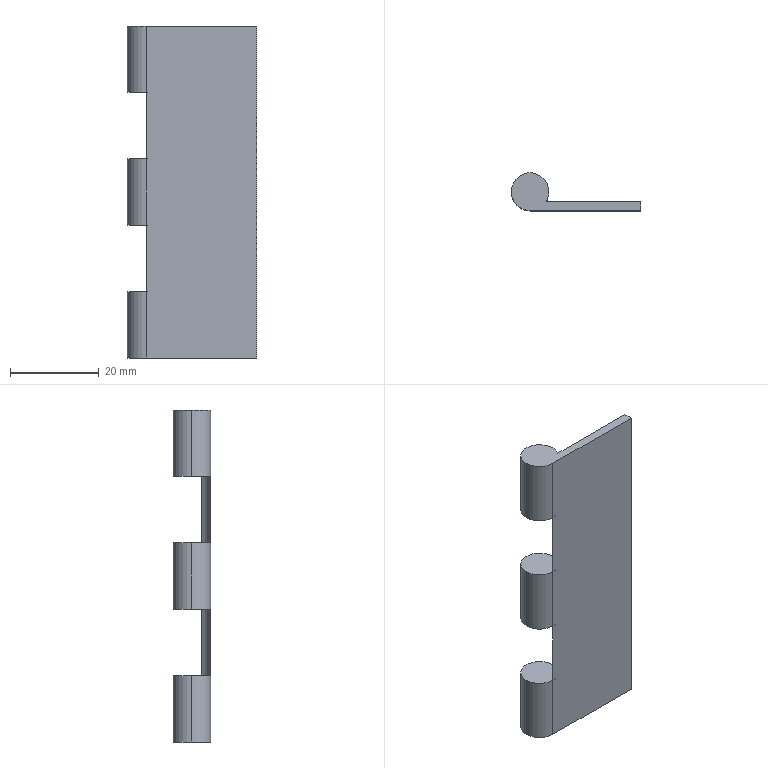Part | STEP file | _PDHFA1-75.step | 1 solid | 20 faces | box 29.25 x 8.5 x 75 mm | volume 5922 mm3 | cylinder 11 | plane 9 | commonest cylinder face diameters 8.5 x11
STEP:
#1=CARTESIAN_POINT('',(0.,0.,0.));
#2=DIRECTION('',(0.,0.,1.));
#3=DIRECTION('',(1.,0.,0.));
#4=AXIS2_PLACEMENT_3D('',#1,#2,#3);
#5=CARTESIAN_POINT('',(3.606,2.,60.));
#6=VERTEX_POINT('',#5);
#7=CARTESIAN_POINT('',(4.25,4.25,60.));
#8=VERTEX_POINT('',#7);
#9=CARTESIAN_POINT('',(0.,4.25,60.));
#10=DIRECTION('',(0.,0.,1.));
#11=DIRECTION('',(1.,0.,0.));
#12=AXIS2_PLACEMENT_3D('',#9,#10,#11);
#13=CIRCLE('',#12,4.25);
#14=CARTESIAN_POINT('',(0.,4.25,75.));
#15=DIRECTION('',(0.,0.,1.));
#16=DIRECTION('',(-1.,0.,0.));
#17=AXIS2_PLACEMENT_3D('',#14,#15,#16);
#18=CYLINDRICAL_SURFACE('',#17,4.25);
#19=CARTESIAN_POINT('',(-3.142,-15.));
#20=DIRECTION('',(1.,0.));
#21=VECTOR('',#20,1.);
#22=LINE('',#19,#21);
#23=(GEOMETRIC_REPRESENTATION_CONTEXT(2)PARAMETRIC_REPRESENTATION_CONTEXT()REPRESENTATION_CONTEXT('',''));
#24=DEFINITIONAL_REPRESENTATION('',(#22),#23);
#25=PCURVE('',#18,#24);
#26=CARTESIAN_POINT('',(0.,4.25,60.));
#27=DIRECTION('',(0.,0.,1.));
#28=DIRECTION('',(1.,0.,0.));
#29=AXIS2_PLACEMENT_3D('',#26,#27,#28);
#30=PLANE('',#29);
#31=CARTESIAN_POINT('',(0.,0.));
#32=DIRECTION('',(1.,0.));
#33=AXIS2_PLACEMENT_2D('',#31,#32);
#34=CIRCLE('',#33,4.25);
#35=(GEOMETRIC_REPRESENTATION_CONTEXT(2)PARAMETRIC_REPRESENTATION_CONTEXT()REPRESENTATION_CONTEXT('',''));
#36=DEFINITIONAL_REPRESENTATION('',(#34),#35);
#37=PCURVE('',#30,#36);
#38=SURFACE_CURVE('',#13,(#25,#37),.PCURVE_S1.);
#39=EDGE_CURVE('',#6,#8,#38,.T.);
#40=ORIENTED_EDGE('',*,*,#39,.T.);
#41=CARTESIAN_POINT('',(4.25,4.25,75.));
#42=VERTEX_POINT('',#41);
#43=CARTESIAN_POINT('',(4.25,4.25,75.));
#44=DIRECTION('',(0.,0.,1.));
#45=VECTOR('',#44,1.);
#46=LINE('',#43,#45);
#47=CARTESIAN_POINT('',(3.142,0.));
#48=DIRECTION('',(0.,1.));
#49=VECTOR('',#48,1.);
#50=LINE('',#47,#49);
#51=(GEOMETRIC_REPRESENTATION_CONTEXT(2)PARAMETRIC_REPRESENTATION_CONTEXT()REPRESENTATION_CONTEXT('',''));
#52=DEFINITIONAL_REPRESENTATION('',(#50),#51);
#53=PCURVE('',#18,#52);
#54=CARTESIAN_POINT('',(0.,4.25,75.));
#55=DIRECTION('',(0.,0.,1.));
#56=DIRECTION('',(-1.,0.,0.));
#57=AXIS2_PLACEMENT_3D('',#54,#55,#56);
#58=CYLINDRICAL_SURFACE('',#57,4.25);
#59=CARTESIAN_POINT('',(3.142,0.));
#60=DIRECTION('',(0.,1.));
#61=VECTOR('',#60,1.);
#62=LINE('',#59,#61);
#63=(GEOMETRIC_REPRESENTATION_CONTEXT(2)PARAMETRIC_REPRESENTATION_CONTEXT()REPRESENTATION_CONTEXT('',''));
#64=DEFINITIONAL_REPRESENTATION('',(#62),#63);
#65=PCURVE('',#58,#64);
#66=SURFACE_CURVE('',#46,(#53,#65),.PCURVE_S1.);
#67=EDGE_CURVE('',#8,#42,#66,.T.);
#68=ORIENTED_EDGE('',*,*,#67,.T.);
#69=CARTESIAN_POINT('',(3.606,2.,75.));
#70=VERTEX_POINT('',#69);
#71=CARTESIAN_POINT('',(0.,4.25,75.));
#72=DIRECTION('',(0.,0.,1.));
#73=DIRECTION('',(1.,0.,0.));
#74=AXIS2_PLACEMENT_3D('',#71,#72,#73);
#75=CIRCLE('',#74,4.25);
#76=CARTESIAN_POINT('',(-3.142,0.));
#77=DIRECTION('',(1.,0.));
#78=VECTOR('',#77,1.);
#79=LINE('',#76,#78);
#80=(GEOMETRIC_REPRESENTATION_CONTEXT(2)PARAMETRIC_REPRESENTATION_CONTEXT()REPRESENTATION_CONTEXT('',''));
#81=DEFINITIONAL_REPRESENTATION('',(#79),#80);
#82=PCURVE('',#18,#81);
#83=CARTESIAN_POINT('',(0.,4.25,75.));
#84=DIRECTION('',(0.,0.,1.));
#85=DIRECTION('',(1.,0.,0.));
#86=AXIS2_PLACEMENT_3D('',#83,#84,#85);
#87=PLANE('',#86);
#88=CARTESIAN_POINT('',(0.,0.));
#89=DIRECTION('',(1.,0.));
#90=AXIS2_PLACEMENT_2D('',#88,#89);
#91=CIRCLE('',#90,4.25);
#92=(GEOMETRIC_REPRESENTATION_CONTEXT(2)PARAMETRIC_REPRESENTATION_CONTEXT()REPRESENTATION_CONTEXT('',''));
#93=DEFINITIONAL_REPRESENTATION('',(#91),#92);
#94=PCURVE('',#87,#93);
#95=SURFACE_CURVE('',#75,(#82,#94),.PCURVE_S1.);
#96=EDGE_CURVE('',#70,#42,#95,.T.);
#97=ORIENTED_EDGE('',*,*,#96,.F.);
#98=CARTESIAN_POINT('',(3.606,2.,75.));
#99=DIRECTION('',(0.,0.,-1.));
#100=VECTOR('',#99,1.);
#101=LINE('',#98,#100);
#102=CARTESIAN_POINT('',(2.584,0.));
#103=DIRECTION('',(0.,-1.));
#104=VECTOR('',#103,1.);
#105=LINE('',#102,#104);
#106=(GEOMETRIC_REPRESENTATION_CONTEXT(2)PARAMETRIC_REPRESENTATION_CONTEXT()REPRESENTATION_CONTEXT('',''));
#107=DEFINITIONAL_REPRESENTATION('',(#105),#106);
#108=PCURVE('',#18,#107);
#109=CARTESIAN_POINT('',(25.,2.,75.));
#110=DIRECTION('',(0.,-1.,0.));
#111=DIRECTION('',(0.,0.,-1.));
#112=AXIS2_PLACEMENT_3D('',#109,#110,#111);
#113=PLANE('',#112);
#114=CARTESIAN_POINT('',(0.,-21.394));
#115=DIRECTION('',(1.,0.));
#116=VECTOR('',#115,1.);
#117=LINE('',#114,#116);
#118=(GEOMETRIC_REPRESENTATION_CONTEXT(2)PARAMETRIC_REPRESENTATION_CONTEXT()REPRESENTATION_CONTEXT('',''));
#119=DEFINITIONAL_REPRESENTATION('',(#117),#118);
#120=PCURVE('',#113,#119);
#121=SURFACE_CURVE('',#101,(#108,#120),.PCURVE_S1.);
#122=EDGE_CURVE('',#70,#6,#121,.T.);
#123=ORIENTED_EDGE('',*,*,#122,.T.);
#124=EDGE_LOOP('',(#40,#68,#97,#123));
#125=FACE_BOUND('',#124,.T.);
#126=ADVANCED_FACE('',(#125),#18,.T.);
#127=ORIENTED_EDGE('',*,*,#67,.F.);
#128=CARTESIAN_POINT('',(-4.25,4.25,60.));
#129=VERTEX_POINT('',#128);
#130=CARTESIAN_POINT('',(0.,4.25,60.));
#131=DIRECTION('',(0.,0.,1.));
#132=DIRECTION('',(1.,0.,0.));
#133=AXIS2_PLACEMENT_3D('',#130,#131,#132);
#134=CIRCLE('',#133,4.25);
#135=CARTESIAN_POINT('',(3.142,-15.));
#136=DIRECTION('',(1.,0.));
#137=VECTOR('',#136,1.);
#138=LINE('',#135,#137);
#139=(GEOMETRIC_REPRESENTATION_CONTEXT(2)PARAMETRIC_REPRESENTATION_CONTEXT()REPRESENTATION_CONTEXT('',''));
#140=DEFINITIONAL_REPRESENTATION('',(#138),#139);
#141=PCURVE('',#58,#140);
#142=CARTESIAN_POINT('',(0.,0.));
#143=DIRECTION('',(1.,0.));
#144=AXIS2_PLACEMENT_2D('',#142,#143);
#145=CIRCLE('',#144,4.25);
#146=(GEOMETRIC_REPRESENTATION_CONTEXT(2)PARAMETRIC_REPRESENTATION_CONTEXT()REPRESENTATION_CONTEXT('',''));
#147=DEFINITIONAL_REPRESENTATION('',(#145),#146);
#148=PCURVE('',#30,#147);
#149=SURFACE_CURVE('',#134,(#141,#148),.PCURVE_S1.);
#150=EDGE_CURVE('',#8,#129,#149,.T.);
#151=ORIENTED_EDGE('',*,*,#150,.T.);
#152=CARTESIAN_POINT('',(-4.25,4.25,75.));
#153=VERTEX_POINT('',#152);
#154=CARTESIAN_POINT('',(-4.25,4.25,75.));
#155=DIRECTION('',(0.,0.,1.));
#156=VECTOR('',#155,1.);
#157=LINE('',#154,#156);
#158=CARTESIAN_POINT('',(6.283,0.));
#159=DIRECTION('',(0.,1.));
#160=VECTOR('',#159,1.);
#161=LINE('',#158,#160);
#162=(GEOMETRIC_REPRESENTATION_CONTEXT(2)PARAMETRIC_REPRESENTATION_CONTEXT()REPRESENTATION_CONTEXT('',''));
#163=DEFINITIONAL_REPRESENTATION('',(#161),#162);
#164=PCURVE('',#58,#163);
#165=CARTESIAN_POINT('',(0.,4.25,75.));
#166=DIRECTION('',(0.,0.,1.));
#167=DIRECTION('',(-1.,0.,0.));
#168=AXIS2_PLACEMENT_3D('',#165,#166,#167);
#169=CYLINDRICAL_SURFACE('',#168,4.25);
#170=CARTESIAN_POINT('',(0.,0.));
#171=DIRECTION('',(0.,1.));
#172=VECTOR('',#171,1.);
#173=LINE('',#170,#172);
#174=(GEOMETRIC_REPRESENTATION_CONTEXT(2)PARAMETRIC_REPRESENTATION_CONTEXT()REPRESENTATION_CONTEXT('',''));
#175=DEFINITIONAL_REPRESENTATION('',(#173),#174);
#176=PCURVE('',#169,#175);
#177=SURFACE_CURVE('',#157,(#164,#176),.PCURVE_S1.);
#178=EDGE_CURVE('',#129,#153,#177,.T.);
#179=ORIENTED_EDGE('',*,*,#178,.T.);
#180=CARTESIAN_POINT('',(0.,4.25,75.));
#181=DIRECTION('',(0.,0.,1.));
#182=DIRECTION('',(1.,0.,0.));
#183=AXIS2_PLACEMENT_3D('',#180,#181,#182);
#184=CIRCLE('',#183,4.25);
#185=CARTESIAN_POINT('',(3.142,0.));
#186=DIRECTION('',(1.,0.));
#187=VECTOR('',#186,1.);
#188=LINE('',#185,#187);
#189=(GEOMETRIC_REPRESENTATION_CONTEXT(2)PARAMETRIC_REPRESENTATION_CONTEXT()REPRESENTATION_CONTEXT('',''));
#190=DEFINITIONAL_REPRESENTATION('',(#188),#189);
#191=PCURVE('',#58,#190);
#192=CARTESIAN_POINT('',(0.,0.));
#193=DIRECTION('',(1.,0.));
#194=AXIS2_PLACEMENT_2D('',#192,#193);
#195=CIRCLE('',#194,4.25);
#196=(GEOMETRIC_REPRESENTATION_CONTEXT(2)PARAMETRIC_REPRESENTATION_CONTEXT()REPRESENTATION_CONTEXT('',''));
#197=DEFINITIONAL_REPRESENTATION('',(#195),#196);
#198=PCURVE('',#87,#197);
#199=SURFACE_CURVE('',#184,(#191,#198),.PCURVE_S1.);
#200=EDGE_CURVE('',#42,#153,#199,.T.);
#201=ORIENTED_EDGE('',*,*,#200,.F.);
#202=EDGE_LOOP('',(#127,#151,#179,#201));
#203=FACE_BOUND('',#202,.T.);
#204=ADVANCED_FACE('',(#203),#58,.T.);
#205=CARTESIAN_POINT('',(3.606,2.,0.));
#206=VERTEX_POINT('',#205);
#207=CARTESIAN_POINT('',(4.25,4.25,0.));
#208=VERTEX_POINT('',#207);
#209=CARTESIAN_POINT('',(0.,4.25,0.));
#210=DIRECTION('',(0.,0.,1.));
#211=DIRECTION('',(1.,0.,0.));
#212=AXIS2_PLACEMENT_3D('',#209,#210,#211);
#213=CIRCLE('',#212,4.25);
#214=CARTESIAN_POINT('',(0.,4.25,75.));
#215=DIRECTION('',(0.,0.,1.));
#216=DIRECTION('',(-1.,0.,0.));
#217=AXIS2_PLACEMENT_3D('',#214,#215,#216);
#218=CYLINDRICAL_SURFACE('',#217,4.25);
#219=CARTESIAN_POINT('',(-3.142,-75.));
#220=DIRECTION('',(1.,0.));
#221=VECTOR('',#220,1.);
#222=LINE('',#219,#221);
#223=(GEOMETRIC_REPRESENTATION_CONTEXT(2)PARAMETRIC_REPRESENTATION_CONTEXT()REPRESENTATION_CONTEXT('',''));
#224=DEFINITIONAL_REPRESENTATION('',(#222),#223);
#225=PCURVE('',#218,#224);
#226=CARTESIAN_POINT('',(0.,4.25,0.));
#227=DIRECTION('',(0.,0.,1.));
#228=DIRECTION('',(1.,0.,0.));
#229=AXIS2_PLACEMENT_3D('',#226,#227,#228);
#230=PLANE('',#229);
#231=CARTESIAN_POINT('',(0.,0.));
#232=DIRECTION('',(1.,0.));
#233=AXIS2_PLACEMENT_2D('',#231,#232);
#234=CIRCLE('',#233,4.25);
#235=(GEOMETRIC_REPRESENTATION_CONTEXT(2)PARAMETRIC_REPRESENTATION_CONTEXT()REPRESENTATION_CONTEXT('',''));
#236=DEFINITIONAL_REPRESENTATION('',(#234),#235);
#237=PCURVE('',#230,#236);
#238=SURFACE_CURVE('',#213,(#225,#237),.PCURVE_S1.);
#239=EDGE_CURVE('',#206,#208,#238,.T.);
#240=ORIENTED_EDGE('',*,*,#239,.T.);
#241=CARTESIAN_POINT('',(4.25,4.25,15.));
#242=VERTEX_POINT('',#241);
#243=CARTESIAN_POINT('',(4.25,4.25,75.));
#244=DIRECTION('',(0.,0.,1.));
#245=VECTOR('',#244,1.);
#246=LINE('',#243,#245);
#247=CARTESIAN_POINT('',(3.142,0.));
#248=DIRECTION('',(0.,1.));
#249=VECTOR('',#248,1.);
#250=LINE('',#247,#249);
#251=(GEOMETRIC_REPRESENTATION_CONTEXT(2)PARAMETRIC_REPRESENTATION_CONTEXT()REPRESENTATION_CONTEXT('',''));
#252=DEFINITIONAL_REPRESENTATION('',(#250),#251);
#253=PCURVE('',#218,#252);
#254=CARTESIAN_POINT('',(0.,4.25,75.));
#255=DIRECTION('',(0.,0.,1.));
#256=DIRECTION('',(-1.,0.,0.));
#257=AXIS2_PLACEMENT_3D('',#254,#255,#256);
#258=CYLINDRICAL_SURFACE('',#257,4.25);
#259=CARTESIAN_POINT('',(3.142,0.));
#260=DIRECTION('',(0.,1.));
#261=VECTOR('',#260,1.);
#262=LINE('',#259,#261);
#263=(GEOMETRIC_REPRESENTATION_CONTEXT(2)PARAMETRIC_REPRESENTATION_CONTEXT()REPRESENTATION_CONTEXT('',''));
#264=DEFINITIONAL_REPRESENTATION('',(#262),#263);
#265=PCURVE('',#258,#264);
#266=SURFACE_CURVE('',#246,(#253,#265),.PCURVE_S1.);
#267=EDGE_CURVE('',#208,#242,#266,.T.);
#268=ORIENTED_EDGE('',*,*,#267,.T.);
#269=CARTESIAN_POINT('',(3.606,2.,15.));
#270=VERTEX_POINT('',#269);
#271=CARTESIAN_POINT('',(0.,4.25,15.));
#272=DIRECTION('',(0.,0.,1.));
#273=DIRECTION('',(1.,0.,0.));
#274=AXIS2_PLACEMENT_3D('',#271,#272,#273);
#275=CIRCLE('',#274,4.25);
#276=CARTESIAN_POINT('',(-3.142,-60.));
#277=DIRECTION('',(1.,0.));
#278=VECTOR('',#277,1.);
#279=LINE('',#276,#278);
#280=(GEOMETRIC_REPRESENTATION_CONTEXT(2)PARAMETRIC_REPRESENTATION_CONTEXT()REPRESENTATION_CONTEXT('',''));
#281=DEFINITIONAL_REPRESENTATION('',(#279),#280);
#282=PCURVE('',#218,#281);
#283=CARTESIAN_POINT('',(0.,4.25,15.));
#284=DIRECTION('',(0.,0.,1.));
#285=DIRECTION('',(1.,0.,0.));
#286=AXIS2_PLACEMENT_3D('',#283,#284,#285);
#287=PLANE('',#286);
#288=CARTESIAN_POINT('',(0.,0.));
#289=DIRECTION('',(1.,0.));
#290=AXIS2_PLACEMENT_2D('',#288,#289);
#291=CIRCLE('',#290,4.25);
#292=(GEOMETRIC_REPRESENTATION_CONTEXT(2)PARAMETRIC_REPRESENTATION_CONTEXT()REPRESENTATION_CONTEXT('',''));
#293=DEFINITIONAL_REPRESENTATION('',(#291),#292);
#294=PCURVE('',#287,#293);
#295=SURFACE_CURVE('',#275,(#282,#294),.PCURVE_S1.);
#296=EDGE_CURVE('',#270,#242,#295,.T.);
#297=ORIENTED_EDGE('',*,*,#296,.F.);
#298=CARTESIAN_POINT('',(3.606,2.,75.));
#299=DIRECTION('',(0.,0.,-1.));
#300=VECTOR('',#299,1.);
#301=LINE('',#298,#300);
#302=CARTESIAN_POINT('',(2.584,0.));
#303=DIRECTION('',(0.,-1.));
#304=VECTOR('',#303,1.);
#305=LINE('',#302,#304);
#306=(GEOMETRIC_REPRESENTATION_CONTEXT(2)PARAMETRIC_REPRESENTATION_CONTEXT()REPRESENTATION_CONTEXT('',''));
#307=DEFINITIONAL_REPRESENTATION('',(#305),#306);
#308=PCURVE('',#218,#307);
#309=CARTESIAN_POINT('',(0.,-21.394));
#310=DIRECTION('',(1.,0.));
#311=VECTOR('',#310,1.);
#312=LINE('',#309,#311);
#313=(GEOMETRIC_REPRESENTATION_CONTEXT(2)PARAMETRIC_REPRESENTATION_CONTEXT()REPRESENTATION_CONTEXT('',''));
#314=DEFINITIONAL_REPRESENTATION('',(#312),#313);
#315=PCURVE('',#113,#314);
#316=SURFACE_CURVE('',#301,(#308,#315),.PCURVE_S1.);
#317=EDGE_CURVE('',#270,#206,#316,.T.);
#318=ORIENTED_EDGE('',*,*,#317,.T.);
#319=EDGE_LOOP('',(#240,#268,#297,#318));
#320=FACE_BOUND('',#319,.T.);
#321=ADVANCED_FACE('',(#320),#218,.T.);
#322=ORIENTED_EDGE('',*,*,#267,.F.);
#323=CARTESIAN_POINT('',(-4.25,4.25,0.));
#324=VERTEX_POINT('',#323);
#325=CARTESIAN_POINT('',(0.,4.25,0.));
#326=DIRECTION('',(0.,0.,1.));
#327=DIRECTION('',(1.,0.,0.));
#328=AXIS2_PLACEMENT_3D('',#325,#326,#327);
#329=CIRCLE('',#328,4.25);
#330=CARTESIAN_POINT('',(3.142,-75.));
#331=DIRECTION('',(1.,0.));
#332=VECTOR('',#331,1.);
#333=LINE('',#330,#332);
#334=(GEOMETRIC_REPRESENTATION_CONTEXT(2)PARAMETRIC_REPRESENTATION_CONTEXT()REPRESENTATION_CONTEXT('',''));
#335=DEFINITIONAL_REPRESENTATION('',(#333),#334);
#336=PCURVE('',#258,#335);
#337=CARTESIAN_POINT('',(0.,0.));
#338=DIRECTION('',(1.,0.));
#339=AXIS2_PLACEMENT_2D('',#337,#338);
#340=CIRCLE('',#339,4.25);
#341=(GEOMETRIC_REPRESENTATION_CONTEXT(2)PARAMETRIC_REPRESENTATION_CONTEXT()REPRESENTATION_CONTEXT('',''));
#342=DEFINITIONAL_REPRESENTATION('',(#340),#341);
#343=PCURVE('',#230,#342);
#344=SURFACE_CURVE('',#329,(#336,#343),.PCURVE_S1.);
#345=EDGE_CURVE('',#208,#324,#344,.T.);
#346=ORIENTED_EDGE('',*,*,#345,.T.);
#347=CARTESIAN_POINT('',(-4.25,4.25,15.));
#348=VERTEX_POINT('',#347);
#349=CARTESIAN_POINT('',(-4.25,4.25,75.));
#350=DIRECTION('',(0.,0.,1.));
#351=VECTOR('',#350,1.);
#352=LINE('',#349,#351);
#353=CARTESIAN_POINT('',(6.283,0.));
#354=DIRECTION('',(0.,1.));
#355=VECTOR('',#354,1.);
#356=LINE('',#353,#355);
#357=(GEOMETRIC_REPRESENTATION_CONTEXT(2)PARAMETRIC_REPRESENTATION_CONTEXT()REPRESENTATION_CONTEXT('',''));
#358=DEFINITIONAL_REPRESENTATION('',(#356),#357);
#359=PCURVE('',#258,#358);
#360=CARTESIAN_POINT('',(0.,4.25,75.));
#361=DIRECTION('',(0.,0.,1.));
#362=DIRECTION('',(-1.,0.,0.));
#363=AXIS2_PLACEMENT_3D('',#360,#361,#362);
#364=CYLINDRICAL_SURFACE('',#363,4.25);
#365=CARTESIAN_POINT('',(0.,0.));
#366=DIRECTION('',(0.,1.));
#367=VECTOR('',#366,1.);
#368=LINE('',#365,#367);
#369=(GEOMETRIC_REPRESENTATION_CONTEXT(2)PARAMETRIC_REPRESENTATION_CONTEXT()REPRESENTATION_CONTEXT('',''));
#370=DEFINITIONAL_REPRESENTATION('',(#368),#369);
#371=PCURVE('',#364,#370);
#372=SURFACE_CURVE('',#352,(#359,#371),.PCURVE_S1.);
#373=EDGE_CURVE('',#324,#348,#372,.T.);
#374=ORIENTED_EDGE('',*,*,#373,.T.);
#375=CARTESIAN_POINT('',(0.,4.25,15.));
#376=DIRECTION('',(0.,0.,1.));
#377=DIRECTION('',(1.,0.,0.));
#378=AXIS2_PLACEMENT_3D('',#375,#376,#377);
#379=CIRCLE('',#378,4.25);
#380=CARTESIAN_POINT('',(3.142,-60.));
#381=DIRECTION('',(1.,0.));
#382=VECTOR('',#381,1.);
#383=LINE('',#380,#382);
#384=(GEOMETRIC_REPRESENTATION_CONTEXT(2)PARAMETRIC_REPRESENTATION_CONTEXT()REPRESENTATION_CONTEXT('',''));
#385=DEFINITIONAL_REPRESENTATION('',(#383),#384);
#386=PCURVE('',#258,#385);
#387=CARTESIAN_POINT('',(0.,0.));
#388=DIRECTION('',(1.,0.));
#389=AXIS2_PLACEMENT_2D('',#387,#388);
#390=CIRCLE('',#389,4.25);
#391=(GEOMETRIC_REPRESENTATION_CONTEXT(2)PARAMETRIC_REPRESENTATION_CONTEXT()REPRESENTATION_CONTEXT('',''));
#392=DEFINITIONAL_REPRESENTATION('',(#390),#391);
#393=PCURVE('',#287,#392);
#394=SURFACE_CURVE('',#379,(#386,#393),.PCURVE_S1.);
#395=EDGE_CURVE('',#242,#348,#394,.T.);
#396=ORIENTED_EDGE('',*,*,#395,.F.);
#397=EDGE_LOOP('',(#322,#346,#374,#396));
#398=FACE_BOUND('',#397,.T.);
#399=ADVANCED_FACE('',(#398),#258,.T.);
#400=CARTESIAN_POINT('',(3.606,2.,30.));
#401=VERTEX_POINT('',#400);
#402=CARTESIAN_POINT('',(4.25,4.25,30.));
#403=VERTEX_POINT('',#402);
#404=CARTESIAN_POINT('',(0.,4.25,30.));
#405=DIRECTION('',(0.,0.,1.));
#406=DIRECTION('',(1.,0.,0.));
#407=AXIS2_PLACEMENT_3D('',#404,#405,#406);
#408=CIRCLE('',#407,4.25);
#409=CARTESIAN_POINT('',(0.,4.25,75.));
#410=DIRECTION('',(0.,0.,1.));
#411=DIRECTION('',(-1.,0.,0.));
#412=AXIS2_PLACEMENT_3D('',#409,#410,#411);
#413=CYLINDRICAL_SURFACE('',#412,4.25);
#414=CARTESIAN_POINT('',(-3.142,-45.));
#415=DIRECTION('',(1.,0.));
#416=VECTOR('',#415,1.);
#417=LINE('',#414,#416);
#418=(GEOMETRIC_REPRESENTATION_CONTEXT(2)PARAMETRIC_REPRESENTATION_CONTEXT()REPRESENTATION_CONTEXT('',''));
#419=DEFINITIONAL_REPRESENTATION('',(#417),#418);
#420=PCURVE('',#413,#419);
#421=CARTESIAN_POINT('',(0.,4.25,30.));
#422=DIRECTION('',(0.,0.,1.));
#423=DIRECTION('',(1.,0.,0.));
#424=AXIS2_PLACEMENT_3D('',#421,#422,#423);
#425=PLANE('',#424);
#426=CARTESIAN_POINT('',(0.,0.));
#427=DIRECTION('',(1.,0.));
#428=AXIS2_PLACEMENT_2D('',#426,#427);
#429=CIRCLE('',#428,4.25);
#430=(GEOMETRIC_REPRESENTATION_CONTEXT(2)PARAMETRIC_REPRESENTATION_CONTEXT()REPRESENTATION_CONTEXT('',''));
#431=DEFINITIONAL_REPRESENTATION('',(#429),#430);
#432=PCURVE('',#425,#431);
#433=SURFACE_CURVE('',#408,(#420,#432),.PCURVE_S1.);
#434=EDGE_CURVE('',#401,#403,#433,.T.);
#435=ORIENTED_EDGE('',*,*,#434,.T.);
#436=CARTESIAN_POINT('',(4.25,4.25,45.));
#437=VERTEX_POINT('',#436);
#438=CARTESIAN_POINT('',(4.25,4.25,75.));
#439=DIRECTION('',(0.,0.,1.));
#440=VECTOR('',#439,1.);
#441=LINE('',#438,#440);
#442=CARTESIAN_POINT('',(3.142,0.));
#443=DIRECTION('',(0.,1.));
#444=VECTOR('',#443,1.);
#445=LINE('',#442,#444);
#446=(GEOMETRIC_REPRESENTATION_CONTEXT(2)PARAMETRIC_REPRESENTATION_CONTEXT()REPRESENTATION_CONTEXT('',''));
#447=DEFINITIONAL_REPRESENTATION('',(#445),#446);
#448=PCURVE('',#413,#447);
#449=CARTESIAN_POINT('',(0.,4.25,75.));
#450=DIRECTION('',(0.,0.,1.));
#451=DIRECTION('',(-1.,0.,0.));
#452=AXIS2_PLACEMENT_3D('',#449,#450,#451);
#453=CYLINDRICAL_SURFACE('',#452,4.25);
#454=CARTESIAN_POINT('',(3.142,0.));
#455=DIRECTION('',(0.,1.));
#456=VECTOR('',#455,1.);
#457=LINE('',#454,#456);
#458=(GEOMETRIC_REPRESENTATION_CONTEXT(2)PARAMETRIC_REPRESENTATION_CONTEXT()REPRESENTATION_CONTEXT('',''));
#459=DEFINITIONAL_REPRESENTATION('',(#457),#458);
#460=PCURVE('',#453,#459);
#461=SURFACE_CURVE('',#441,(#448,#460),.PCURVE_S1.);
#462=EDGE_CURVE('',#403,#437,#461,.T.);
#463=ORIENTED_EDGE('',*,*,#462,.T.);
#464=CARTESIAN_POINT('',(3.606,2.,45.));
#465=VERTEX_POINT('',#464);
#466=CARTESIAN_POINT('',(0.,4.25,45.));
#467=DIRECTION('',(0.,0.,1.));
#468=DIRECTION('',(1.,0.,0.));
#469=AXIS2_PLACEMENT_3D('',#466,#467,#468);
#470=CIRCLE('',#469,4.25);
#471=CARTESIAN_POINT('',(-3.142,-30.));
#472=DIRECTION('',(1.,0.));
#473=VECTOR('',#472,1.);
#474=LINE('',#471,#473);
#475=(GEOMETRIC_REPRESENTATION_CONTEXT(2)PARAMETRIC_REPRESENTATION_CONTEXT()REPRESENTATION_CONTEXT('',''));
#476=DEFINITIONAL_REPRESENTATION('',(#474),#475);
#477=PCURVE('',#413,#476);
#478=CARTESIAN_POINT('',(0.,4.25,45.));
#479=DIRECTION('',(0.,0.,1.));
#480=DIRECTION('',(1.,0.,0.));
#481=AXIS2_PLACEMENT_3D('',#478,#479,#480);
#482=PLANE('',#481);
#483=CARTESIAN_POINT('',(0.,0.));
#484=DIRECTION('',(1.,0.));
#485=AXIS2_PLACEMENT_2D('',#483,#484);
#486=CIRCLE('',#485,4.25);
#487=(GEOMETRIC_REPRESENTATION_CONTEXT(2)PARAMETRIC_REPRESENTATION_CONTEXT()REPRESENTATION_CONTEXT('',''));
#488=DEFINITIONAL_REPRESENTATION('',(#486),#487);
#489=PCURVE('',#482,#488);
#490=SURFACE_CURVE('',#470,(#477,#489),.PCURVE_S1.);
#491=EDGE_CURVE('',#465,#437,#490,.T.);
#492=ORIENTED_EDGE('',*,*,#491,.F.);
#493=CARTESIAN_POINT('',(3.606,2.,75.));
#494=DIRECTION('',(0.,0.,-1.));
#495=VECTOR('',#494,1.);
#496=LINE('',#493,#495);
#497=CARTESIAN_POINT('',(2.584,0.));
#498=DIRECTION('',(0.,-1.));
#499=VECTOR('',#498,1.);
#500=LINE('',#497,#499);
#501=(GEOMETRIC_REPRESENTATION_CONTEXT(2)PARAMETRIC_REPRESENTATION_CONTEXT()REPRESENTATION_CONTEXT('',''));
#502=DEFINITIONAL_REPRESENTATION('',(#500),#501);
#503=PCURVE('',#413,#502);
#504=CARTESIAN_POINT('',(0.,-21.394));
#505=DIRECTION('',(1.,0.));
#506=VECTOR('',#505,1.);
#507=LINE('',#504,#506);
#508=(GEOMETRIC_REPRESENTATION_CONTEXT(2)PARAMETRIC_REPRESENTATION_CONTEXT()REPRESENTATION_CONTEXT('',''));
#509=DEFINITIONAL_REPRESENTATION('',(#507),#508);
#510=PCURVE('',#113,#509);
#511=SURFACE_CURVE('',#496,(#503,#510),.PCURVE_S1.);
#512=EDGE_CURVE('',#465,#401,#511,.T.);
#513=ORIENTED_EDGE('',*,*,#512,.T.);
#514=EDGE_LOOP('',(#435,#463,#492,#513));
#515=FACE_BOUND('',#514,.T.);
#516=ADVANCED_FACE('',(#515),#413,.T.);
#517=ORIENTED_EDGE('',*,*,#462,.F.);
#518=CARTESIAN_POINT('',(-4.25,4.25,30.));
#519=VERTEX_POINT('',#518);
#520=CARTESIAN_POINT('',(0.,4.25,30.));
#521=DIRECTION('',(0.,0.,1.));
#522=DIRECTION('',(1.,0.,0.));
#523=AXIS2_PLACEMENT_3D('',#520,#521,#522);
#524=CIRCLE('',#523,4.25);
#525=CARTESIAN_POINT('',(3.142,-45.));
#526=DIRECTION('',(1.,0.));
#527=VECTOR('',#526,1.);
#528=LINE('',#525,#527);
#529=(GEOMETRIC_REPRESENTATION_CONTEXT(2)PARAMETRIC_REPRESENTATION_CONTEXT()REPRESENTATION_CONTEXT('',''));
#530=DEFINITIONAL_REPRESENTATION('',(#528),#529);
#531=PCURVE('',#453,#530);
#532=CARTESIAN_POINT('',(0.,0.));
#533=DIRECTION('',(1.,0.));
#534=AXIS2_PLACEMENT_2D('',#532,#533);
#535=CIRCLE('',#534,4.25);
#536=(GEOMETRIC_REPRESENTATION_CONTEXT(2)PARAMETRIC_REPRESENTATION_CONTEXT()REPRESENTATION_CONTEXT('',''));
#537=DEFINITIONAL_REPRESENTATION('',(#535),#536);
#538=PCURVE('',#425,#537);
#539=SURFACE_CURVE('',#524,(#531,#538),.PCURVE_S1.);
#540=EDGE_CURVE('',#403,#519,#539,.T.);
#541=ORIENTED_EDGE('',*,*,#540,.T.);
#542=CARTESIAN_POINT('',(-4.25,4.25,45.));
#543=VERTEX_POINT('',#542);
#544=CARTESIAN_POINT('',(-4.25,4.25,75.));
#545=DIRECTION('',(0.,0.,1.));
#546=VECTOR('',#545,1.);
#547=LINE('',#544,#546);
#548=CARTESIAN_POINT('',(6.283,0.));
#549=DIRECTION('',(0.,1.));
#550=VECTOR('',#549,1.);
#551=LINE('',#548,#550);
#552=(GEOMETRIC_REPRESENTATION_CONTEXT(2)PARAMETRIC_REPRESENTATION_CONTEXT()REPRESENTATION_CONTEXT('',''));
#553=DEFINITIONAL_REPRESENTATION('',(#551),#552);
#554=PCURVE('',#453,#553);
#555=CARTESIAN_POINT('',(0.,4.25,75.));
#556=DIRECTION('',(0.,0.,1.));
#557=DIRECTION('',(-1.,0.,0.));
#558=AXIS2_PLACEMENT_3D('',#555,#556,#557);
#559=CYLINDRICAL_SURFACE('',#558,4.25);
#560=CARTESIAN_POINT('',(0.,0.));
#561=DIRECTION('',(0.,1.));
#562=VECTOR('',#561,1.);
#563=LINE('',#560,#562);
#564=(GEOMETRIC_REPRESENTATION_CONTEXT(2)PARAMETRIC_REPRESENTATION_CONTEXT()REPRESENTATION_CONTEXT('',''));
#565=DEFINITIONAL_REPRESENTATION('',(#563),#564);
#566=PCURVE('',#559,#565);
#567=SURFACE_CURVE('',#547,(#554,#566),.PCURVE_S1.);
#568=EDGE_CURVE('',#519,#543,#567,.T.);
#569=ORIENTED_EDGE('',*,*,#568,.T.);
#570=CARTESIAN_POINT('',(0.,4.25,45.));
#571=DIRECTION('',(0.,0.,1.));
#572=DIRECTION('',(1.,0.,0.));
#573=AXIS2_PLACEMENT_3D('',#570,#571,#572);
#574=CIRCLE('',#573,4.25);
#575=CARTESIAN_POINT('',(3.142,-30.));
#576=DIRECTION('',(1.,0.));
#577=VECTOR('',#576,1.);
#578=LINE('',#575,#577);
#579=(GEOMETRIC_REPRESENTATION_CONTEXT(2)PARAMETRIC_REPRESENTATION_CONTEXT()REPRESENTATION_CONTEXT('',''));
#580=DEFINITIONAL_REPRESENTATION('',(#578),#579);
#581=PCURVE('',#453,#580);
#582=CARTESIAN_POINT('',(0.,0.));
#583=DIRECTION('',(1.,0.));
#584=AXIS2_PLACEMENT_2D('',#582,#583);
#585=CIRCLE('',#584,4.25);
#586=(GEOMETRIC_REPRESENTATION_CONTEXT(2)PARAMETRIC_REPRESENTATION_CONTEXT()REPRESENTATION_CONTEXT('',''));
#587=DEFINITIONAL_REPRESENTATION('',(#585),#586);
#588=PCURVE('',#482,#587);
#589=SURFACE_CURVE('',#574,(#581,#588),.PCURVE_S1.);
#590=EDGE_CURVE('',#437,#543,#589,.T.);
#591=ORIENTED_EDGE('',*,*,#590,.F.);
#592=EDGE_LOOP('',(#517,#541,#569,#591));
#593=FACE_BOUND('',#592,.T.);
#594=ADVANCED_FACE('',(#593),#453,.T.);
#595=CARTESIAN_POINT('',(0.,0.,60.));
#596=VERTEX_POINT('',#595);
#597=CARTESIAN_POINT('',(0.,4.25,60.));
#598=DIRECTION('',(0.,0.,1.));
#599=DIRECTION('',(1.,0.,0.));
#600=AXIS2_PLACEMENT_3D('',#597,#598,#599);
#601=CIRCLE('',#600,4.25);
#602=CARTESIAN_POINT('',(0.,0.));
#603=DIRECTION('',(1.,0.));
#604=AXIS2_PLACEMENT_2D('',#602,#603);
#605=CIRCLE('',#604,4.25);
#606=(GEOMETRIC_REPRESENTATION_CONTEXT(2)PARAMETRIC_REPRESENTATION_CONTEXT()REPRESENTATION_CONTEXT('',''));
#607=DEFINITIONAL_REPRESENTATION('',(#605),#606);
#608=PCURVE('',#30,#607);
#609=CARTESIAN_POINT('',(0.,4.25,60.));
#610=DIRECTION('',(0.,0.,1.));
#611=DIRECTION('',(-1.,0.,0.));
#612=AXIS2_PLACEMENT_3D('',#609,#610,#611);
#613=CYLINDRICAL_SURFACE('',#612,4.25);
#614=CARTESIAN_POINT('',(-3.142,0.));
#615=DIRECTION('',(1.,0.));
#616=VECTOR('',#615,1.);
#617=LINE('',#614,#616);
#618=(GEOMETRIC_REPRESENTATION_CONTEXT(2)PARAMETRIC_REPRESENTATION_CONTEXT()REPRESENTATION_CONTEXT('',''));
#619=DEFINITIONAL_REPRESENTATION('',(#617),#618);
#620=PCURVE('',#613,#619);
#621=SURFACE_CURVE('',#601,(#608,#620),.PCURVE_S1.);
#622=EDGE_CURVE('',#596,#6,#621,.T.);
#623=ORIENTED_EDGE('',*,*,#622,.F.);
#624=CARTESIAN_POINT('',(0.,4.25,60.));
#625=DIRECTION('',(0.,0.,1.));
#626=DIRECTION('',(1.,0.,0.));
#627=AXIS2_PLACEMENT_3D('',#624,#625,#626);
#628=CIRCLE('',#627,4.25);
#629=CARTESIAN_POINT('',(0.,0.));
#630=DIRECTION('',(1.,0.));
#631=AXIS2_PLACEMENT_2D('',#629,#630);
#632=CIRCLE('',#631,4.25);
#633=(GEOMETRIC_REPRESENTATION_CONTEXT(2)PARAMETRIC_REPRESENTATION_CONTEXT()REPRESENTATION_CONTEXT('',''));
#634=DEFINITIONAL_REPRESENTATION('',(#632),#633);
#635=PCURVE('',#30,#634);
#636=CARTESIAN_POINT('',(-3.142,-15.));
#637=DIRECTION('',(1.,0.));
#638=VECTOR('',#637,1.);
#639=LINE('',#636,#638);
#640=(GEOMETRIC_REPRESENTATION_CONTEXT(2)PARAMETRIC_REPRESENTATION_CONTEXT()REPRESENTATION_CONTEXT('',''));
#641=DEFINITIONAL_REPRESENTATION('',(#639),#640);
#642=PCURVE('',#169,#641);
#643=SURFACE_CURVE('',#628,(#635,#642),.PCURVE_S1.);
#644=EDGE_CURVE('',#129,#596,#643,.T.);
#645=ORIENTED_EDGE('',*,*,#644,.F.);
#646=ORIENTED_EDGE('',*,*,#150,.F.);
#647=ORIENTED_EDGE('',*,*,#39,.F.);
#648=EDGE_LOOP('',(#623,#645,#646,#647));
#649=FACE_BOUND('',#648,.T.);
#650=ADVANCED_FACE('',(#649),#30,.F.);
#651=CARTESIAN_POINT('',(0.,0.,45.));
#652=VERTEX_POINT('',#651);
#653=CARTESIAN_POINT('',(0.,4.25,45.));
#654=DIRECTION('',(0.,0.,1.));
#655=DIRECTION('',(1.,0.,0.));
#656=AXIS2_PLACEMENT_3D('',#653,#654,#655);
#657=CIRCLE('',#656,4.25);
#658=CARTESIAN_POINT('',(0.,0.));
#659=DIRECTION('',(1.,0.));
#660=AXIS2_PLACEMENT_2D('',#658,#659);
#661=CIRCLE('',#660,4.25);
#662=(GEOMETRIC_REPRESENTATION_CONTEXT(2)PARAMETRIC_REPRESENTATION_CONTEXT()REPRESENTATION_CONTEXT('',''));
#663=DEFINITIONAL_REPRESENTATION('',(#661),#662);
#664=PCURVE('',#482,#663);
#665=CARTESIAN_POINT('',(-3.142,-15.));
#666=DIRECTION('',(1.,0.));
#667=VECTOR('',#666,1.);
#668=LINE('',#665,#667);
#669=(GEOMETRIC_REPRESENTATION_CONTEXT(2)PARAMETRIC_REPRESENTATION_CONTEXT()REPRESENTATION_CONTEXT('',''));
#670=DEFINITIONAL_REPRESENTATION('',(#668),#669);
#671=PCURVE('',#613,#670);
#672=SURFACE_CURVE('',#657,(#664,#671),.PCURVE_S1.);
#673=EDGE_CURVE('',#652,#465,#672,.T.);
#674=ORIENTED_EDGE('',*,*,#673,.T.);
#675=ORIENTED_EDGE('',*,*,#491,.T.);
#676=ORIENTED_EDGE('',*,*,#590,.T.);
#677=CARTESIAN_POINT('',(0.,4.25,45.));
#678=DIRECTION('',(0.,0.,1.));
#679=DIRECTION('',(1.,0.,0.));
#680=AXIS2_PLACEMENT_3D('',#677,#678,#679);
#681=CIRCLE('',#680,4.25);
#682=CARTESIAN_POINT('',(0.,0.));
#683=DIRECTION('',(1.,0.));
#684=AXIS2_PLACEMENT_2D('',#682,#683);
#685=CIRCLE('',#684,4.25);
#686=(GEOMETRIC_REPRESENTATION_CONTEXT(2)PARAMETRIC_REPRESENTATION_CONTEXT()REPRESENTATION_CONTEXT('',''));
#687=DEFINITIONAL_REPRESENTATION('',(#685),#686);
#688=PCURVE('',#482,#687);
#689=CARTESIAN_POINT('',(-3.142,-30.));
#690=DIRECTION('',(1.,0.));
#691=VECTOR('',#690,1.);
#692=LINE('',#689,#691);
#693=(GEOMETRIC_REPRESENTATION_CONTEXT(2)PARAMETRIC_REPRESENTATION_CONTEXT()REPRESENTATION_CONTEXT('',''));
#694=DEFINITIONAL_REPRESENTATION('',(#692),#693);
#695=PCURVE('',#559,#694);
#696=SURFACE_CURVE('',#681,(#688,#695),.PCURVE_S1.);
#697=EDGE_CURVE('',#543,#652,#696,.T.);
#698=ORIENTED_EDGE('',*,*,#697,.T.);
#699=EDGE_LOOP('',(#674,#675,#676,#698));
#700=FACE_BOUND('',#699,.T.);
#701=ADVANCED_FACE('',(#700),#482,.T.);
#702=ORIENTED_EDGE('',*,*,#622,.F.);
#703=CARTESIAN_POINT('',(0.,0.,75.));
#704=DIRECTION('',(0.,0.,-1.));
#705=VECTOR('',#704,1.);
#706=LINE('',#703,#705);
#707=CARTESIAN_POINT('',(1.571,15.));
#708=DIRECTION('',(0.,-1.));
#709=VECTOR('',#708,1.);
#710=LINE('',#707,#709);
#711=(GEOMETRIC_REPRESENTATION_CONTEXT(2)PARAMETRIC_REPRESENTATION_CONTEXT()REPRESENTATION_CONTEXT('',''));
#712=DEFINITIONAL_REPRESENTATION('',(#710),#711);
#713=PCURVE('',#613,#712);
#714=CARTESIAN_POINT('',(0.,0.,75.));
#715=DIRECTION('',(0.,1.,0.));
#716=DIRECTION('',(1.,0.,0.));
#717=AXIS2_PLACEMENT_3D('',#714,#715,#716);
#718=PLANE('',#717);
#719=CARTESIAN_POINT('',(0.,0.));
#720=DIRECTION('',(0.,1.));
#721=VECTOR('',#720,1.);
#722=LINE('',#719,#721);
#723=(GEOMETRIC_REPRESENTATION_CONTEXT(2)PARAMETRIC_REPRESENTATION_CONTEXT()REPRESENTATION_CONTEXT('',''));
#724=DEFINITIONAL_REPRESENTATION('',(#722),#723);
#725=PCURVE('',#718,#724);
#726=SURFACE_CURVE('',#706,(#713,#725),.PCURVE_S1.);
#727=EDGE_CURVE('',#596,#652,#726,.T.);
#728=ORIENTED_EDGE('',*,*,#727,.T.);
#729=ORIENTED_EDGE('',*,*,#673,.T.);
#730=CARTESIAN_POINT('',(3.606,2.,60.));
#731=DIRECTION('',(0.,0.,-1.));
#732=VECTOR('',#731,1.);
#733=LINE('',#730,#732);
#734=CARTESIAN_POINT('',(2.584,0.));
#735=DIRECTION('',(0.,-1.));
#736=VECTOR('',#735,1.);
#737=LINE('',#734,#736);
#738=(GEOMETRIC_REPRESENTATION_CONTEXT(2)PARAMETRIC_REPRESENTATION_CONTEXT()REPRESENTATION_CONTEXT('',''));
#739=DEFINITIONAL_REPRESENTATION('',(#737),#738);
#740=PCURVE('',#613,#739);
#741=CARTESIAN_POINT('',(15.,-21.394));
#742=DIRECTION('',(1.,0.));
#743=VECTOR('',#742,1.);
#744=LINE('',#741,#743);
#745=(GEOMETRIC_REPRESENTATION_CONTEXT(2)PARAMETRIC_REPRESENTATION_CONTEXT()REPRESENTATION_CONTEXT('',''));
#746=DEFINITIONAL_REPRESENTATION('',(#744),#745);
#747=PCURVE('',#113,#746);
#748=SURFACE_CURVE('',#733,(#740,#747),.PCURVE_S1.);
#749=EDGE_CURVE('',#6,#465,#748,.T.);
#750=ORIENTED_EDGE('',*,*,#749,.F.);
#751=EDGE_LOOP('',(#702,#728,#729,#750));
#752=FACE_BOUND('',#751,.F.);
#753=ADVANCED_FACE('',(#752),#613,.F.);
#754=ORIENTED_EDGE('',*,*,#568,.F.);
#755=CARTESIAN_POINT('',(0.,0.,30.));
#756=VERTEX_POINT('',#755);
#757=CARTESIAN_POINT('',(0.,4.25,30.));
#758=DIRECTION('',(0.,0.,1.));
#759=DIRECTION('',(1.,0.,0.));
#760=AXIS2_PLACEMENT_3D('',#757,#758,#759);
#761=CIRCLE('',#760,4.25);
#762=CARTESIAN_POINT('',(-3.142,-45.));
#763=DIRECTION('',(1.,0.));
#764=VECTOR('',#763,1.);
#765=LINE('',#762,#764);
#766=(GEOMETRIC_REPRESENTATION_CONTEXT(2)PARAMETRIC_REPRESENTATION_CONTEXT()REPRESENTATION_CONTEXT('',''));
#767=DEFINITIONAL_REPRESENTATION('',(#765),#766);
#768=PCURVE('',#559,#767);
#769=CARTESIAN_POINT('',(0.,0.));
#770=DIRECTION('',(1.,0.));
#771=AXIS2_PLACEMENT_2D('',#769,#770);
#772=CIRCLE('',#771,4.25);
#773=(GEOMETRIC_REPRESENTATION_CONTEXT(2)PARAMETRIC_REPRESENTATION_CONTEXT()REPRESENTATION_CONTEXT('',''));
#774=DEFINITIONAL_REPRESENTATION('',(#772),#773);
#775=PCURVE('',#425,#774);
#776=SURFACE_CURVE('',#761,(#768,#775),.PCURVE_S1.);
#777=EDGE_CURVE('',#519,#756,#776,.T.);
#778=ORIENTED_EDGE('',*,*,#777,.T.);
#779=CARTESIAN_POINT('',(0.,0.,75.));
#780=DIRECTION('',(0.,0.,-1.));
#781=VECTOR('',#780,1.);
#782=LINE('',#779,#781);
#783=CARTESIAN_POINT('',(1.571,0.));
#784=DIRECTION('',(0.,-1.));
#785=VECTOR('',#784,1.);
#786=LINE('',#783,#785);
#787=(GEOMETRIC_REPRESENTATION_CONTEXT(2)PARAMETRIC_REPRESENTATION_CONTEXT()REPRESENTATION_CONTEXT('',''));
#788=DEFINITIONAL_REPRESENTATION('',(#786),#787);
#789=PCURVE('',#559,#788);
#790=CARTESIAN_POINT('',(0.,0.));
#791=DIRECTION('',(0.,1.));
#792=VECTOR('',#791,1.);
#793=LINE('',#790,#792);
#794=(GEOMETRIC_REPRESENTATION_CONTEXT(2)PARAMETRIC_REPRESENTATION_CONTEXT()REPRESENTATION_CONTEXT('',''));
#795=DEFINITIONAL_REPRESENTATION('',(#793),#794);
#796=PCURVE('',#718,#795);
#797=SURFACE_CURVE('',#782,(#789,#796),.PCURVE_S1.);
#798=EDGE_CURVE('',#652,#756,#797,.T.);
#799=ORIENTED_EDGE('',*,*,#798,.F.);
#800=ORIENTED_EDGE('',*,*,#697,.F.);
#801=EDGE_LOOP('',(#754,#778,#799,#800));
#802=FACE_BOUND('',#801,.T.);
#803=ADVANCED_FACE('',(#802),#559,.T.);
#804=ORIENTED_EDGE('',*,*,#373,.F.);
#805=CARTESIAN_POINT('',(0.,0.,0.));
#806=VERTEX_POINT('',#805);
#807=CARTESIAN_POINT('',(0.,4.25,0.));
#808=DIRECTION('',(0.,0.,1.));
#809=DIRECTION('',(1.,0.,0.));
#810=AXIS2_PLACEMENT_3D('',#807,#808,#809);
#811=CIRCLE('',#810,4.25);
#812=CARTESIAN_POINT('',(-3.142,-75.));
#813=DIRECTION('',(1.,0.));
#814=VECTOR('',#813,1.);
#815=LINE('',#812,#814);
#816=(GEOMETRIC_REPRESENTATION_CONTEXT(2)PARAMETRIC_REPRESENTATION_CONTEXT()REPRESENTATION_CONTEXT('',''));
#817=DEFINITIONAL_REPRESENTATION('',(#815),#816);
#818=PCURVE('',#364,#817);
#819=CARTESIAN_POINT('',(0.,0.));
#820=DIRECTION('',(1.,0.));
#821=AXIS2_PLACEMENT_2D('',#819,#820);
#822=CIRCLE('',#821,4.25);
#823=(GEOMETRIC_REPRESENTATION_CONTEXT(2)PARAMETRIC_REPRESENTATION_CONTEXT()REPRESENTATION_CONTEXT('',''));
#824=DEFINITIONAL_REPRESENTATION('',(#822),#823);
#825=PCURVE('',#230,#824);
#826=SURFACE_CURVE('',#811,(#818,#825),.PCURVE_S1.);
#827=EDGE_CURVE('',#324,#806,#826,.T.);
#828=ORIENTED_EDGE('',*,*,#827,.T.);
#829=CARTESIAN_POINT('',(0.,0.,15.));
#830=VERTEX_POINT('',#829);
#831=CARTESIAN_POINT('',(0.,0.,75.));
#832=DIRECTION('',(0.,0.,-1.));
#833=VECTOR('',#832,1.);
#834=LINE('',#831,#833);
#835=CARTESIAN_POINT('',(1.571,0.));
#836=DIRECTION('',(0.,-1.));
#837=VECTOR('',#836,1.);
#838=LINE('',#835,#837);
#839=(GEOMETRIC_REPRESENTATION_CONTEXT(2)PARAMETRIC_REPRESENTATION_CONTEXT()REPRESENTATION_CONTEXT('',''));
#840=DEFINITIONAL_REPRESENTATION('',(#838),#839);
#841=PCURVE('',#364,#840);
#842=CARTESIAN_POINT('',(0.,0.));
#843=DIRECTION('',(0.,1.));
#844=VECTOR('',#843,1.);
#845=LINE('',#842,#844);
#846=(GEOMETRIC_REPRESENTATION_CONTEXT(2)PARAMETRIC_REPRESENTATION_CONTEXT()REPRESENTATION_CONTEXT('',''));
#847=DEFINITIONAL_REPRESENTATION('',(#845),#846);
#848=PCURVE('',#718,#847);
#849=SURFACE_CURVE('',#834,(#841,#848),.PCURVE_S1.);
#850=EDGE_CURVE('',#830,#806,#849,.T.);
#851=ORIENTED_EDGE('',*,*,#850,.F.);
#852=CARTESIAN_POINT('',(0.,4.25,15.));
#853=DIRECTION('',(0.,0.,1.));
#854=DIRECTION('',(1.,0.,0.));
#855=AXIS2_PLACEMENT_3D('',#852,#853,#854);
#856=CIRCLE('',#855,4.25);
#857=CARTESIAN_POINT('',(-3.142,-60.));
#858=DIRECTION('',(1.,0.));
#859=VECTOR('',#858,1.);
#860=LINE('',#857,#859);
#861=(GEOMETRIC_REPRESENTATION_CONTEXT(2)PARAMETRIC_REPRESENTATION_CONTEXT()REPRESENTATION_CONTEXT('',''));
#862=DEFINITIONAL_REPRESENTATION('',(#860),#861);
#863=PCURVE('',#364,#862);
#864=CARTESIAN_POINT('',(0.,0.));
#865=DIRECTION('',(1.,0.));
#866=AXIS2_PLACEMENT_2D('',#864,#865);
#867=CIRCLE('',#866,4.25);
#868=(GEOMETRIC_REPRESENTATION_CONTEXT(2)PARAMETRIC_REPRESENTATION_CONTEXT()REPRESENTATION_CONTEXT('',''));
#869=DEFINITIONAL_REPRESENTATION('',(#867),#868);
#870=PCURVE('',#287,#869);
#871=SURFACE_CURVE('',#856,(#863,#870),.PCURVE_S1.);
#872=EDGE_CURVE('',#348,#830,#871,.T.);
#873=ORIENTED_EDGE('',*,*,#872,.F.);
#874=EDGE_LOOP('',(#804,#828,#851,#873));
#875=FACE_BOUND('',#874,.T.);
#876=ADVANCED_FACE('',(#875),#364,.T.);
#877=ORIENTED_EDGE('',*,*,#178,.F.);
#878=ORIENTED_EDGE('',*,*,#644,.T.);
#879=CARTESIAN_POINT('',(0.,0.,75.));
#880=VERTEX_POINT('',#879);
#881=CARTESIAN_POINT('',(0.,0.,75.));
#882=DIRECTION('',(0.,0.,-1.));
#883=VECTOR('',#882,1.);
#884=LINE('',#881,#883);
#885=CARTESIAN_POINT('',(1.571,0.));
#886=DIRECTION('',(0.,-1.));
#887=VECTOR('',#886,1.);
#888=LINE('',#885,#887);
#889=(GEOMETRIC_REPRESENTATION_CONTEXT(2)PARAMETRIC_REPRESENTATION_CONTEXT()REPRESENTATION_CONTEXT('',''));
#890=DEFINITIONAL_REPRESENTATION('',(#888),#889);
#891=PCURVE('',#169,#890);
#892=CARTESIAN_POINT('',(0.,0.));
#893=DIRECTION('',(0.,1.));
#894=VECTOR('',#893,1.);
#895=LINE('',#892,#894);
#896=(GEOMETRIC_REPRESENTATION_CONTEXT(2)PARAMETRIC_REPRESENTATION_CONTEXT()REPRESENTATION_CONTEXT('',''));
#897=DEFINITIONAL_REPRESENTATION('',(#895),#896);
#898=PCURVE('',#718,#897);
#899=SURFACE_CURVE('',#884,(#891,#898),.PCURVE_S1.);
#900=EDGE_CURVE('',#880,#596,#899,.T.);
#901=ORIENTED_EDGE('',*,*,#900,.F.);
#902=CARTESIAN_POINT('',(0.,4.25,75.));
#903=DIRECTION('',(0.,0.,1.));
#904=DIRECTION('',(1.,0.,0.));
#905=AXIS2_PLACEMENT_3D('',#902,#903,#904);
#906=CIRCLE('',#905,4.25);
#907=CARTESIAN_POINT('',(-3.142,0.));
#908=DIRECTION('',(1.,0.));
#909=VECTOR('',#908,1.);
#910=LINE('',#907,#909);
#911=(GEOMETRIC_REPRESENTATION_CONTEXT(2)PARAMETRIC_REPRESENTATION_CONTEXT()REPRESENTATION_CONTEXT('',''));
#912=DEFINITIONAL_REPRESENTATION('',(#910),#911);
#913=PCURVE('',#169,#912);
#914=CARTESIAN_POINT('',(0.,0.));
#915=DIRECTION('',(1.,0.));
#916=AXIS2_PLACEMENT_2D('',#914,#915);
#917=CIRCLE('',#916,4.25);
#918=(GEOMETRIC_REPRESENTATION_CONTEXT(2)PARAMETRIC_REPRESENTATION_CONTEXT()REPRESENTATION_CONTEXT('',''));
#919=DEFINITIONAL_REPRESENTATION('',(#917),#918);
#920=PCURVE('',#87,#919);
#921=SURFACE_CURVE('',#906,(#913,#920),.PCURVE_S1.);
#922=EDGE_CURVE('',#153,#880,#921,.T.);
#923=ORIENTED_EDGE('',*,*,#922,.F.);
#924=EDGE_LOOP('',(#877,#878,#901,#923));
#925=FACE_BOUND('',#924,.T.);
#926=ADVANCED_FACE('',(#925),#169,.T.);
#927=CARTESIAN_POINT('',(25.,0.,0.));
#928=VERTEX_POINT('',#927);
#929=CARTESIAN_POINT('',(0.,0.,0.));
#930=DIRECTION('',(1.,0.,0.));
#931=VECTOR('',#930,1.);
#932=LINE('',#929,#931);
#933=CARTESIAN_POINT('',(0.,75.));
#934=DIRECTION('',(1.,0.));
#935=VECTOR('',#934,1.);
#936=LINE('',#933,#935);
#937=(GEOMETRIC_REPRESENTATION_CONTEXT(2)PARAMETRIC_REPRESENTATION_CONTEXT()REPRESENTATION_CONTEXT('',''));
#938=DEFINITIONAL_REPRESENTATION('',(#936),#937);
#939=PCURVE('',#718,#938);
#940=CARTESIAN_POINT('',(0.,-4.25));
#941=DIRECTION('',(1.,0.));
#942=VECTOR('',#941,1.);
#943=LINE('',#940,#942);
#944=(GEOMETRIC_REPRESENTATION_CONTEXT(2)PARAMETRIC_REPRESENTATION_CONTEXT()REPRESENTATION_CONTEXT('',''));
#945=DEFINITIONAL_REPRESENTATION('',(#943),#944);
#946=PCURVE('',#230,#945);
#947=SURFACE_CURVE('',#932,(#939,#946),.PCURVE_S1.);
#948=EDGE_CURVE('',#806,#928,#947,.T.);
#949=ORIENTED_EDGE('',*,*,#948,.T.);
#950=CARTESIAN_POINT('',(25.,0.,75.));
#951=VERTEX_POINT('',#950);
#952=CARTESIAN_POINT('',(25.,0.,75.));
#953=DIRECTION('',(0.,0.,-1.));
#954=VECTOR('',#953,1.);
#955=LINE('',#952,#954);
#956=CARTESIAN_POINT('',(25.,0.));
#957=DIRECTION('',(0.,1.));
#958=VECTOR('',#957,1.);
#959=LINE('',#956,#958);
#960=(GEOMETRIC_REPRESENTATION_CONTEXT(2)PARAMETRIC_REPRESENTATION_CONTEXT()REPRESENTATION_CONTEXT('',''));
#961=DEFINITIONAL_REPRESENTATION('',(#959),#960);
#962=PCURVE('',#718,#961);
#963=CARTESIAN_POINT('',(25.,0.,75.));
#964=DIRECTION('',(-1.,0.,0.));
#965=DIRECTION('',(0.,0.,1.));
#966=AXIS2_PLACEMENT_3D('',#963,#964,#965);
#967=PLANE('',#966);
#968=CARTESIAN_POINT('',(0.,0.));
#969=DIRECTION('',(-1.,0.));
#970=VECTOR('',#969,1.);
#971=LINE('',#968,#970);
#972=(GEOMETRIC_REPRESENTATION_CONTEXT(2)PARAMETRIC_REPRESENTATION_CONTEXT()REPRESENTATION_CONTEXT('',''));
#973=DEFINITIONAL_REPRESENTATION('',(#971),#972);
#974=PCURVE('',#967,#973);
#975=SURFACE_CURVE('',#955,(#962,#974),.PCURVE_S1.);
#976=EDGE_CURVE('',#951,#928,#975,.T.);
#977=ORIENTED_EDGE('',*,*,#976,.F.);
#978=CARTESIAN_POINT('',(0.,0.,75.));
#979=DIRECTION('',(1.,0.,0.));
#980=VECTOR('',#979,1.);
#981=LINE('',#978,#980);
#982=CARTESIAN_POINT('',(0.,0.));
#983=DIRECTION('',(1.,0.));
#984=VECTOR('',#983,1.);
#985=LINE('',#982,#984);
#986=(GEOMETRIC_REPRESENTATION_CONTEXT(2)PARAMETRIC_REPRESENTATION_CONTEXT()REPRESENTATION_CONTEXT('',''));
#987=DEFINITIONAL_REPRESENTATION('',(#985),#986);
#988=PCURVE('',#718,#987);
#989=CARTESIAN_POINT('',(0.,-4.25));
#990=DIRECTION('',(1.,0.));
#991=VECTOR('',#990,1.);
#992=LINE('',#989,#991);
#993=(GEOMETRIC_REPRESENTATION_CONTEXT(2)PARAMETRIC_REPRESENTATION_CONTEXT()REPRESENTATION_CONTEXT('',''));
#994=DEFINITIONAL_REPRESENTATION('',(#992),#993);
#995=PCURVE('',#87,#994);
#996=SURFACE_CURVE('',#981,(#988,#995),.PCURVE_S1.);
#997=EDGE_CURVE('',#880,#951,#996,.T.);
#998=ORIENTED_EDGE('',*,*,#997,.F.);
#999=ORIENTED_EDGE('',*,*,#900,.T.);
#1000=ORIENTED_EDGE('',*,*,#727,.T.);
#1001=ORIENTED_EDGE('',*,*,#798,.T.);
#1002=CARTESIAN_POINT('',(0.,0.,75.));
#1003=DIRECTION('',(0.,0.,-1.));
#1004=VECTOR('',#1003,1.);
#1005=LINE('',#1002,#1004);
#1006=CARTESIAN_POINT('',(0.,0.));
#1007=DIRECTION('',(0.,1.));
#1008=VECTOR('',#1007,1.);
#1009=LINE('',#1006,#1008);
#1010=(GEOMETRIC_REPRESENTATION_CONTEXT(2)PARAMETRIC_REPRESENTATION_CONTEXT()REPRESENTATION_CONTEXT('',''));
#1011=DEFINITIONAL_REPRESENTATION('',(#1009),#1010);
#1012=PCURVE('',#718,#1011);
#1013=CARTESIAN_POINT('',(0.,4.25,30.));
#1014=DIRECTION('',(0.,0.,1.));
#1015=DIRECTION('',(-1.,0.,0.));
#1016=AXIS2_PLACEMENT_3D('',#1013,#1014,#1015);
#1017=CYLINDRICAL_SURFACE('',#1016,4.25);
#1018=CARTESIAN_POINT('',(1.571,45.));
#1019=DIRECTION('',(0.,-1.));
#1020=VECTOR('',#1019,1.);
#1021=LINE('',#1018,#1020);
#1022=(GEOMETRIC_REPRESENTATION_CONTEXT(2)PARAMETRIC_REPRESENTATION_CONTEXT()REPRESENTATION_CONTEXT('',''));
#1023=DEFINITIONAL_REPRESENTATION('',(#1021),#1022);
#1024=PCURVE('',#1017,#1023);
#1025=SURFACE_CURVE('',#1005,(#1012,#1024),.PCURVE_S1.);
#1026=EDGE_CURVE('',#756,#830,#1025,.T.);
#1027=ORIENTED_EDGE('',*,*,#1026,.T.);
#1028=ORIENTED_EDGE('',*,*,#850,.T.);
#1029=EDGE_LOOP('',(#949,#977,#998,#999,#1000,#1001,#1027,#1028));
#1030=FACE_BOUND('',#1029,.T.);
#1031=ADVANCED_FACE('',(#1030),#718,.F.);
#1032=CARTESIAN_POINT('',(25.,2.,0.));
#1033=VERTEX_POINT('',#1032);
#1034=CARTESIAN_POINT('',(25.,2.,0.));
#1035=DIRECTION('',(-1.,0.,0.));
#1036=VECTOR('',#1035,1.);
#1037=LINE('',#1034,#1036);
#1038=CARTESIAN_POINT('',(75.,0.));
#1039=DIRECTION('',(0.,-1.));
#1040=VECTOR('',#1039,1.);
#1041=LINE('',#1038,#1040);
#1042=(GEOMETRIC_REPRESENTATION_CONTEXT(2)PARAMETRIC_REPRESENTATION_CONTEXT()REPRESENTATION_CONTEXT('',''));
#1043=DEFINITIONAL_REPRESENTATION('',(#1041),#1042);
#1044=PCURVE('',#113,#1043);
#1045=CARTESIAN_POINT('',(25.,-2.25));
#1046=DIRECTION('',(-1.,0.));
#1047=VECTOR('',#1046,1.);
#1048=LINE('',#1045,#1047);
#1049=(GEOMETRIC_REPRESENTATION_CONTEXT(2)PARAMETRIC_REPRESENTATION_CONTEXT()REPRESENTATION_CONTEXT('',''));
#1050=DEFINITIONAL_REPRESENTATION('',(#1048),#1049);
#1051=PCURVE('',#230,#1050);
#1052=SURFACE_CURVE('',#1037,(#1044,#1051),.PCURVE_S1.);
#1053=EDGE_CURVE('',#1033,#206,#1052,.T.);
#1054=ORIENTED_EDGE('',*,*,#1053,.T.);
#1055=ORIENTED_EDGE('',*,*,#317,.F.);
#1056=CARTESIAN_POINT('',(3.606,2.,30.));
#1057=DIRECTION('',(0.,0.,-1.));
#1058=VECTOR('',#1057,1.);
#1059=LINE('',#1056,#1058);
#1060=CARTESIAN_POINT('',(45.,-21.394));
#1061=DIRECTION('',(1.,0.));
#1062=VECTOR('',#1061,1.);
#1063=LINE('',#1060,#1062);
#1064=(GEOMETRIC_REPRESENTATION_CONTEXT(2)PARAMETRIC_REPRESENTATION_CONTEXT()REPRESENTATION_CONTEXT('',''));
#1065=DEFINITIONAL_REPRESENTATION('',(#1063),#1064);
#1066=PCURVE('',#113,#1065);
#1067=CARTESIAN_POINT('',(2.584,0.));
#1068=DIRECTION('',(0.,-1.));
#1069=VECTOR('',#1068,1.);
#1070=LINE('',#1067,#1069);
#1071=(GEOMETRIC_REPRESENTATION_CONTEXT(2)PARAMETRIC_REPRESENTATION_CONTEXT()REPRESENTATION_CONTEXT('',''));
#1072=DEFINITIONAL_REPRESENTATION('',(#1070),#1071);
#1073=PCURVE('',#1017,#1072);
#1074=SURFACE_CURVE('',#1059,(#1066,#1073),.PCURVE_S1.);
#1075=EDGE_CURVE('',#401,#270,#1074,.T.);
#1076=ORIENTED_EDGE('',*,*,#1075,.F.);
#1077=ORIENTED_EDGE('',*,*,#512,.F.);
#1078=ORIENTED_EDGE('',*,*,#749,.F.);
#1079=ORIENTED_EDGE('',*,*,#122,.F.);
#1080=CARTESIAN_POINT('',(25.,2.,75.));
#1081=VERTEX_POINT('',#1080);
#1082=CARTESIAN_POINT('',(25.,2.,75.));
#1083=DIRECTION('',(-1.,0.,0.));
#1084=VECTOR('',#1083,1.);
#1085=LINE('',#1082,#1084);
#1086=CARTESIAN_POINT('',(0.,0.));
#1087=DIRECTION('',(0.,-1.));
#1088=VECTOR('',#1087,1.);
#1089=LINE('',#1086,#1088);
#1090=(GEOMETRIC_REPRESENTATION_CONTEXT(2)PARAMETRIC_REPRESENTATION_CONTEXT()REPRESENTATION_CONTEXT('',''));
#1091=DEFINITIONAL_REPRESENTATION('',(#1089),#1090);
#1092=PCURVE('',#113,#1091);
#1093=CARTESIAN_POINT('',(25.,-2.25));
#1094=DIRECTION('',(-1.,0.));
#1095=VECTOR('',#1094,1.);
#1096=LINE('',#1093,#1095);
#1097=(GEOMETRIC_REPRESENTATION_CONTEXT(2)PARAMETRIC_REPRESENTATION_CONTEXT()REPRESENTATION_CONTEXT('',''));
#1098=DEFINITIONAL_REPRESENTATION('',(#1096),#1097);
#1099=PCURVE('',#87,#1098);
#1100=SURFACE_CURVE('',#1085,(#1092,#1099),.PCURVE_S1.);
#1101=EDGE_CURVE('',#1081,#70,#1100,.T.);
#1102=ORIENTED_EDGE('',*,*,#1101,.F.);
#1103=CARTESIAN_POINT('',(25.,2.,75.));
#1104=DIRECTION('',(0.,0.,-1.));
#1105=VECTOR('',#1104,1.);
#1106=LINE('',#1103,#1105);
#1107=CARTESIAN_POINT('',(0.,0.));
#1108=DIRECTION('',(1.,0.));
#1109=VECTOR('',#1108,1.);
#1110=LINE('',#1107,#1109);
#1111=(GEOMETRIC_REPRESENTATION_CONTEXT(2)PARAMETRIC_REPRESENTATION_CONTEXT()REPRESENTATION_CONTEXT('',''));
#1112=DEFINITIONAL_REPRESENTATION('',(#1110),#1111);
#1113=PCURVE('',#113,#1112);
#1114=CARTESIAN_POINT('',(0.,2.));
#1115=DIRECTION('',(-1.,0.));
#1116=VECTOR('',#1115,1.);
#1117=LINE('',#1114,#1116);
#1118=(GEOMETRIC_REPRESENTATION_CONTEXT(2)PARAMETRIC_REPRESENTATION_CONTEXT()REPRESENTATION_CONTEXT('',''));
#1119=DEFINITIONAL_REPRESENTATION('',(#1117),#1118);
#1120=PCURVE('',#967,#1119);
#1121=SURFACE_CURVE('',#1106,(#1113,#1120),.PCURVE_S1.);
#1122=EDGE_CURVE('',#1081,#1033,#1121,.T.);
#1123=ORIENTED_EDGE('',*,*,#1122,.T.);
#1124=EDGE_LOOP('',(#1054,#1055,#1076,#1077,#1078,#1079,#1102,#1123));
#1125=FACE_BOUND('',#1124,.T.);
#1126=ADVANCED_FACE('',(#1125),#113,.F.);
#1127=CARTESIAN_POINT('',(25.,0.,0.));
#1128=DIRECTION('',(0.,1.,0.));
#1129=VECTOR('',#1128,1.);
#1130=LINE('',#1127,#1129);
#1131=CARTESIAN_POINT('',(-75.,0.));
#1132=DIRECTION('',(0.,1.));
#1133=VECTOR('',#1132,1.);
#1134=LINE('',#1131,#1133);
#1135=(GEOMETRIC_REPRESENTATION_CONTEXT(2)PARAMETRIC_REPRESENTATION_CONTEXT()REPRESENTATION_CONTEXT('',''));
#1136=DEFINITIONAL_REPRESENTATION('',(#1134),#1135);
#1137=PCURVE('',#967,#1136);
#1138=CARTESIAN_POINT('',(25.,-4.25));
#1139=DIRECTION('',(0.,1.));
#1140=VECTOR('',#1139,1.);
#1141=LINE('',#1138,#1140);
#1142=(GEOMETRIC_REPRESENTATION_CONTEXT(2)PARAMETRIC_REPRESENTATION_CONTEXT()REPRESENTATION_CONTEXT('',''));
#1143=DEFINITIONAL_REPRESENTATION('',(#1141),#1142);
#1144=PCURVE('',#230,#1143);
#1145=SURFACE_CURVE('',#1130,(#1137,#1144),.PCURVE_S1.);
#1146=EDGE_CURVE('',#928,#1033,#1145,.T.);
#1147=ORIENTED_EDGE('',*,*,#1146,.T.);
#1148=ORIENTED_EDGE('',*,*,#1122,.F.);
#1149=CARTESIAN_POINT('',(25.,0.,75.));
#1150=DIRECTION('',(0.,1.,0.));
#1151=VECTOR('',#1150,1.);
#1152=LINE('',#1149,#1151);
#1153=CARTESIAN_POINT('',(0.,0.));
#1154=DIRECTION('',(0.,1.));
#1155=VECTOR('',#1154,1.);
#1156=LINE('',#1153,#1155);
#1157=(GEOMETRIC_REPRESENTATION_CONTEXT(2)PARAMETRIC_REPRESENTATION_CONTEXT()REPRESENTATION_CONTEXT('',''));
#1158=DEFINITIONAL_REPRESENTATION('',(#1156),#1157);
#1159=PCURVE('',#967,#1158);
#1160=CARTESIAN_POINT('',(25.,-4.25));
#1161=DIRECTION('',(0.,1.));
#1162=VECTOR('',#1161,1.);
#1163=LINE('',#1160,#1162);
#1164=(GEOMETRIC_REPRESENTATION_CONTEXT(2)PARAMETRIC_REPRESENTATION_CONTEXT()REPRESENTATION_CONTEXT('',''));
#1165=DEFINITIONAL_REPRESENTATION('',(#1163),#1164);
#1166=PCURVE('',#87,#1165);
#1167=SURFACE_CURVE('',#1152,(#1159,#1166),.PCURVE_S1.);
#1168=EDGE_CURVE('',#951,#1081,#1167,.T.);
#1169=ORIENTED_EDGE('',*,*,#1168,.F.);
#1170=ORIENTED_EDGE('',*,*,#976,.T.);
#1171=EDGE_LOOP('',(#1147,#1148,#1169,#1170));
#1172=FACE_BOUND('',#1171,.T.);
#1173=ADVANCED_FACE('',(#1172),#967,.F.);
#1174=ORIENTED_EDGE('',*,*,#1053,.F.);
#1175=ORIENTED_EDGE('',*,*,#1146,.F.);
#1176=ORIENTED_EDGE('',*,*,#948,.F.);
#1177=ORIENTED_EDGE('',*,*,#827,.F.);
#1178=ORIENTED_EDGE('',*,*,#345,.F.);
#1179=ORIENTED_EDGE('',*,*,#239,.F.);
#1180=EDGE_LOOP('',(#1174,#1175,#1176,#1177,#1178,#1179));
#1181=FACE_BOUND('',#1180,.T.);
#1182=ADVANCED_FACE('',(#1181),#230,.F.);
#1183=ORIENTED_EDGE('',*,*,#1101,.T.);
#1184=ORIENTED_EDGE('',*,*,#96,.T.);
#1185=ORIENTED_EDGE('',*,*,#200,.T.);
#1186=ORIENTED_EDGE('',*,*,#922,.T.);
#1187=ORIENTED_EDGE('',*,*,#997,.T.);
#1188=ORIENTED_EDGE('',*,*,#1168,.T.);
#1189=EDGE_LOOP('',(#1183,#1184,#1185,#1186,#1187,#1188));
#1190=FACE_BOUND('',#1189,.T.);
#1191=ADVANCED_FACE('',(#1190),#87,.T.);
#1192=CARTESIAN_POINT('',(0.,4.25,30.));
#1193=DIRECTION('',(0.,0.,1.));
#1194=DIRECTION('',(1.,0.,0.));
#1195=AXIS2_PLACEMENT_3D('',#1192,#1193,#1194);
#1196=CIRCLE('',#1195,4.25);
#1197=CARTESIAN_POINT('',(-3.142,0.));
#1198=DIRECTION('',(1.,0.));
#1199=VECTOR('',#1198,1.);
#1200=LINE('',#1197,#1199);
#1201=(GEOMETRIC_REPRESENTATION_CONTEXT(2)PARAMETRIC_REPRESENTATION_CONTEXT()REPRESENTATION_CONTEXT('',''));
#1202=DEFINITIONAL_REPRESENTATION('',(#1200),#1201);
#1203=PCURVE('',#1017,#1202);
#1204=CARTESIAN_POINT('',(0.,0.));
#1205=DIRECTION('',(1.,0.));
#1206=AXIS2_PLACEMENT_2D('',#1204,#1205);
#1207=CIRCLE('',#1206,4.25);
#1208=(GEOMETRIC_REPRESENTATION_CONTEXT(2)PARAMETRIC_REPRESENTATION_CONTEXT()REPRESENTATION_CONTEXT('',''));
#1209=DEFINITIONAL_REPRESENTATION('',(#1207),#1208);
#1210=PCURVE('',#425,#1209);
#1211=SURFACE_CURVE('',#1196,(#1203,#1210),.PCURVE_S1.);
#1212=EDGE_CURVE('',#756,#401,#1211,.T.);
#1213=ORIENTED_EDGE('',*,*,#1212,.F.);
#1214=ORIENTED_EDGE('',*,*,#1026,.T.);
#1215=CARTESIAN_POINT('',(0.,4.25,15.));
#1216=DIRECTION('',(0.,0.,1.));
#1217=DIRECTION('',(1.,0.,0.));
#1218=AXIS2_PLACEMENT_3D('',#1215,#1216,#1217);
#1219=CIRCLE('',#1218,4.25);
#1220=CARTESIAN_POINT('',(-3.142,-15.));
#1221=DIRECTION('',(1.,0.));
#1222=VECTOR('',#1221,1.);
#1223=LINE('',#1220,#1222);
#1224=(GEOMETRIC_REPRESENTATION_CONTEXT(2)PARAMETRIC_REPRESENTATION_CONTEXT()REPRESENTATION_CONTEXT('',''));
#1225=DEFINITIONAL_REPRESENTATION('',(#1223),#1224);
#1226=PCURVE('',#1017,#1225);
#1227=CARTESIAN_POINT('',(0.,0.));
#1228=DIRECTION('',(1.,0.));
#1229=AXIS2_PLACEMENT_2D('',#1227,#1228);
#1230=CIRCLE('',#1229,4.25);
#1231=(GEOMETRIC_REPRESENTATION_CONTEXT(2)PARAMETRIC_REPRESENTATION_CONTEXT()REPRESENTATION_CONTEXT('',''));
#1232=DEFINITIONAL_REPRESENTATION('',(#1230),#1231);
#1233=PCURVE('',#287,#1232);
#1234=SURFACE_CURVE('',#1219,(#1226,#1233),.PCURVE_S1.);
#1235=EDGE_CURVE('',#830,#270,#1234,.T.);
#1236=ORIENTED_EDGE('',*,*,#1235,.T.);
#1237=ORIENTED_EDGE('',*,*,#1075,.F.);
#1238=EDGE_LOOP('',(#1213,#1214,#1236,#1237));
#1239=FACE_BOUND('',#1238,.F.);
#1240=ADVANCED_FACE('',(#1239),#1017,.F.);
#1241=ORIENTED_EDGE('',*,*,#1235,.T.);
#1242=ORIENTED_EDGE('',*,*,#296,.T.);
#1243=ORIENTED_EDGE('',*,*,#395,.T.);
#1244=ORIENTED_EDGE('',*,*,#872,.T.);
#1245=EDGE_LOOP('',(#1241,#1242,#1243,#1244));
#1246=FACE_BOUND('',#1245,.T.);
#1247=ADVANCED_FACE('',(#1246),#287,.T.);
#1248=ORIENTED_EDGE('',*,*,#1212,.F.);
#1249=ORIENTED_EDGE('',*,*,#777,.F.);
#1250=ORIENTED_EDGE('',*,*,#540,.F.);
#1251=ORIENTED_EDGE('',*,*,#434,.F.);
#1252=EDGE_LOOP('',(#1248,#1249,#1250,#1251));
#1253=FACE_BOUND('',#1252,.T.);
#1254=ADVANCED_FACE('',(#1253),#425,.F.);
#1255=CLOSED_SHELL('',(#126,#204,#321,#399,#516,#594,#650,#701,#753,#803,#876,#926,#1031,#1126,#1173,#1182,#1191,#1240,#1247,#1254));
#1256=MANIFOLD_SOLID_BREP('',#1255);
#1257=(LENGTH_UNIT()NAMED_UNIT(*)SI_UNIT(.MILLI.,.METRE.));
#1258=UNCERTAINTY_MEASURE_WITH_UNIT(LENGTH_MEASURE(0.0000001),#1257,'','');
#1259=(NAMED_UNIT(*)PLANE_ANGLE_UNIT()SI_UNIT($,.RADIAN.));
#1260=(NAMED_UNIT(*)SI_UNIT($,.STERADIAN.)SOLID_ANGLE_UNIT());
#1261=(GEOMETRIC_REPRESENTATION_CONTEXT(3)GLOBAL_UNCERTAINTY_ASSIGNED_CONTEXT((#1258))GLOBAL_UNIT_ASSIGNED_CONTEXT((#1257,#1259,#1260))REPRESENTATION_CONTEXT('',''));
#1262=ADVANCED_BREP_SHAPE_REPRESENTATION('',(#4,#1256),#1261);